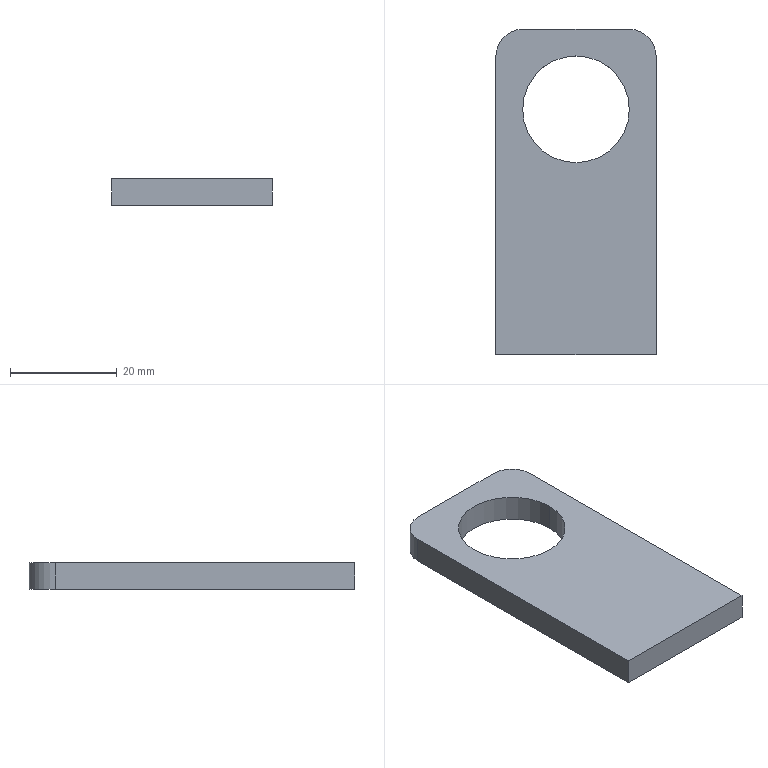Part | SolidWorks | features Extrusion 1, Fillet 1 | 1 solid | 10 faces | box 30 x 61 x 5 mm | volume 7526 mm3 | plane 6 | cylinder 4 | commonest cylinder face diameters 10 x2 20 x2
STEP:
#1=CARTESIAN_POINT('',(-10.,15.5,2.5));
#2=VERTEX_POINT('',#1);
#3=CARTESIAN_POINT('',(10.,15.5,2.5));
#4=VERTEX_POINT('',#3);
#5=CARTESIAN_POINT('',(0.,15.5,2.5));
#6=DIRECTION('',(0.,0.,1.));
#7=DIRECTION('',(1.,0.,0.));
#8=AXIS2_PLACEMENT_3D('',#5,#6,#7);
#9=CIRCLE('',#8,10.);
#10=EDGE_CURVE('',#2,#4,#9,.T.);
#11=ORIENTED_EDGE('',*,*,#10,.T.);
#12=CARTESIAN_POINT('',(10.,15.5,-2.5));
#13=VERTEX_POINT('',#12);
#14=CARTESIAN_POINT('',(10.,15.5,2.5));
#15=DIRECTION('',(0.,0.,-1.));
#16=VECTOR('',#15,1000.);
#17=LINE('',#14,#16);
#18=EDGE_CURVE('',#4,#13,#17,.T.);
#19=ORIENTED_EDGE('',*,*,#18,.T.);
#20=CARTESIAN_POINT('',(-10.,15.5,-2.5));
#21=VERTEX_POINT('',#20);
#22=CARTESIAN_POINT('',(0.,15.5,-2.5));
#23=DIRECTION('',(0.,0.,1.));
#24=DIRECTION('',(1.,0.,0.));
#25=AXIS2_PLACEMENT_3D('',#22,#23,#24);
#26=CIRCLE('',#25,10.);
#27=EDGE_CURVE('',#21,#13,#26,.T.);
#28=ORIENTED_EDGE('',*,*,#27,.F.);
#29=CARTESIAN_POINT('',(-10.,15.5,2.5));
#30=DIRECTION('',(0.,0.,-1.));
#31=VECTOR('',#30,1000.);
#32=LINE('',#29,#31);
#33=EDGE_CURVE('',#2,#21,#32,.T.);
#34=ORIENTED_EDGE('',*,*,#33,.F.);
#35=EDGE_LOOP('',(#11,#19,#28,#34));
#36=FACE_OUTER_BOUND('',#35,.T.);
#37=CARTESIAN_POINT('',(0.,15.5,2.5));
#38=DIRECTION('',(0.,0.,-1.));
#39=DIRECTION('',(-1.,0.,0.));
#40=AXIS2_PLACEMENT_3D('',#37,#38,#39);
#41=CYLINDRICAL_SURFACE('',#40,10.);
#42=ADVANCED_FACE('',(#36),#41,.F.);
#43=CARTESIAN_POINT('',(15.,-30.5,2.5));
#44=VERTEX_POINT('',#43);
#45=CARTESIAN_POINT('',(15.,25.5,2.5));
#46=VERTEX_POINT('',#45);
#47=CARTESIAN_POINT('',(15.,-30.5,2.5));
#48=DIRECTION('',(0.,1.,0.));
#49=VECTOR('',#48,1000.);
#50=LINE('',#47,#49);
#51=EDGE_CURVE('',#44,#46,#50,.T.);
#52=ORIENTED_EDGE('',*,*,#51,.T.);
#53=CARTESIAN_POINT('',(10.,30.5,2.5));
#54=VERTEX_POINT('',#53);
#55=CARTESIAN_POINT('',(10.,25.5,2.5));
#56=DIRECTION('',(0.,0.,1.));
#57=DIRECTION('',(-1.,0.,0.));
#58=AXIS2_PLACEMENT_3D('',#55,#56,#57);
#59=CIRCLE('',#58,5.);
#60=EDGE_CURVE('',#46,#54,#59,.T.);
#61=ORIENTED_EDGE('',*,*,#60,.T.);
#62=CARTESIAN_POINT('',(-10.,30.5,2.5));
#63=VERTEX_POINT('',#62);
#64=CARTESIAN_POINT('',(-15.,30.5,2.5));
#65=DIRECTION('',(-1.,0.,0.));
#66=VECTOR('',#65,1000.);
#67=LINE('',#64,#66);
#68=EDGE_CURVE('',#54,#63,#67,.T.);
#69=ORIENTED_EDGE('',*,*,#68,.T.);
#70=CARTESIAN_POINT('',(-15.,25.5,2.5));
#71=VERTEX_POINT('',#70);
#72=CARTESIAN_POINT('',(-10.,25.5,2.5));
#73=DIRECTION('',(0.,0.,1.));
#74=DIRECTION('',(-1.,0.,0.));
#75=AXIS2_PLACEMENT_3D('',#72,#73,#74);
#76=CIRCLE('',#75,5.);
#77=EDGE_CURVE('',#63,#71,#76,.T.);
#78=ORIENTED_EDGE('',*,*,#77,.T.);
#79=CARTESIAN_POINT('',(-15.,-30.5,2.5));
#80=VERTEX_POINT('',#79);
#81=CARTESIAN_POINT('',(-15.,-30.5,2.5));
#82=DIRECTION('',(0.,-1.,0.));
#83=VECTOR('',#82,1000.);
#84=LINE('',#81,#83);
#85=EDGE_CURVE('',#71,#80,#84,.T.);
#86=ORIENTED_EDGE('',*,*,#85,.T.);
#87=CARTESIAN_POINT('',(-15.,-30.5,2.5));
#88=DIRECTION('',(1.,0.,0.));
#89=VECTOR('',#88,1000.);
#90=LINE('',#87,#89);
#91=EDGE_CURVE('',#80,#44,#90,.T.);
#92=ORIENTED_EDGE('',*,*,#91,.T.);
#93=EDGE_LOOP('',(#52,#61,#69,#78,#86,#92));
#94=FACE_OUTER_BOUND('',#93,.T.);
#95=ORIENTED_EDGE('',*,*,#10,.F.);
#96=CARTESIAN_POINT('',(0.,15.5,2.5));
#97=DIRECTION('',(0.,0.,1.));
#98=DIRECTION('',(1.,0.,0.));
#99=AXIS2_PLACEMENT_3D('',#96,#97,#98);
#100=CIRCLE('',#99,10.);
#101=EDGE_CURVE('',#4,#2,#100,.T.);
#102=ORIENTED_EDGE('',*,*,#101,.F.);
#103=EDGE_LOOP('',(#95,#102));
#104=FACE_BOUND('',#103,.T.);
#105=CARTESIAN_POINT('',(0.,0.,2.5));
#106=DIRECTION('',(0.,0.,-1.));
#107=DIRECTION('',(-1.,0.,0.));
#108=AXIS2_PLACEMENT_3D('',#105,#106,#107);
#109=PLANE('',#108);
#110=ADVANCED_FACE('',(#94,#104),#109,.F.);
#111=CARTESIAN_POINT('',(10.,30.5,-2.5));
#112=VERTEX_POINT('',#111);
#113=CARTESIAN_POINT('',(-10.,30.5,-2.5));
#114=VERTEX_POINT('',#113);
#115=CARTESIAN_POINT('',(-15.,30.5,-2.5));
#116=DIRECTION('',(-1.,0.,0.));
#117=VECTOR('',#116,1000.);
#118=LINE('',#115,#117);
#119=EDGE_CURVE('',#112,#114,#118,.T.);
#120=ORIENTED_EDGE('',*,*,#119,.F.);
#121=CARTESIAN_POINT('',(15.,25.5,-2.5));
#122=VERTEX_POINT('',#121);
#123=CARTESIAN_POINT('',(10.,25.5,-2.5));
#124=DIRECTION('',(0.,0.,-1.));
#125=DIRECTION('',(-1.,0.,0.));
#126=AXIS2_PLACEMENT_3D('',#123,#124,#125);
#127=CIRCLE('',#126,5.);
#128=EDGE_CURVE('',#112,#122,#127,.T.);
#129=ORIENTED_EDGE('',*,*,#128,.T.);
#130=CARTESIAN_POINT('',(15.,-30.5,-2.5));
#131=VERTEX_POINT('',#130);
#132=CARTESIAN_POINT('',(15.,-30.5,-2.5));
#133=DIRECTION('',(0.,1.,0.));
#134=VECTOR('',#133,1000.);
#135=LINE('',#132,#134);
#136=EDGE_CURVE('',#131,#122,#135,.T.);
#137=ORIENTED_EDGE('',*,*,#136,.F.);
#138=CARTESIAN_POINT('',(-15.,-30.5,-2.5));
#139=VERTEX_POINT('',#138);
#140=CARTESIAN_POINT('',(-15.,-30.5,-2.5));
#141=DIRECTION('',(1.,0.,0.));
#142=VECTOR('',#141,1000.);
#143=LINE('',#140,#142);
#144=EDGE_CURVE('',#139,#131,#143,.T.);
#145=ORIENTED_EDGE('',*,*,#144,.F.);
#146=CARTESIAN_POINT('',(-15.,25.5,-2.5));
#147=VERTEX_POINT('',#146);
#148=CARTESIAN_POINT('',(-15.,-30.5,-2.5));
#149=DIRECTION('',(0.,-1.,0.));
#150=VECTOR('',#149,1000.);
#151=LINE('',#148,#150);
#152=EDGE_CURVE('',#147,#139,#151,.T.);
#153=ORIENTED_EDGE('',*,*,#152,.F.);
#154=CARTESIAN_POINT('',(-10.,25.5,-2.5));
#155=DIRECTION('',(0.,0.,-1.));
#156=DIRECTION('',(-1.,0.,0.));
#157=AXIS2_PLACEMENT_3D('',#154,#155,#156);
#158=CIRCLE('',#157,5.);
#159=EDGE_CURVE('',#147,#114,#158,.T.);
#160=ORIENTED_EDGE('',*,*,#159,.T.);
#161=EDGE_LOOP('',(#120,#129,#137,#145,#153,#160));
#162=FACE_OUTER_BOUND('',#161,.T.);
#163=ORIENTED_EDGE('',*,*,#27,.T.);
#164=CARTESIAN_POINT('',(0.,15.5,-2.5));
#165=DIRECTION('',(0.,0.,1.));
#166=DIRECTION('',(1.,0.,0.));
#167=AXIS2_PLACEMENT_3D('',#164,#165,#166);
#168=CIRCLE('',#167,10.);
#169=EDGE_CURVE('',#13,#21,#168,.T.);
#170=ORIENTED_EDGE('',*,*,#169,.T.);
#171=EDGE_LOOP('',(#163,#170));
#172=FACE_BOUND('',#171,.T.);
#173=CARTESIAN_POINT('',(0.,0.,-2.5));
#174=DIRECTION('',(0.,0.,-1.));
#175=DIRECTION('',(-1.,0.,0.));
#176=AXIS2_PLACEMENT_3D('',#173,#174,#175);
#177=PLANE('',#176);
#178=ADVANCED_FACE('',(#162,#172),#177,.T.);
#179=ORIENTED_EDGE('',*,*,#136,.T.);
#180=CARTESIAN_POINT('',(15.,25.5,2.5));
#181=DIRECTION('',(0.,0.,1.));
#182=VECTOR('',#181,1000.);
#183=LINE('',#180,#182);
#184=EDGE_CURVE('',#122,#46,#183,.T.);
#185=ORIENTED_EDGE('',*,*,#184,.T.);
#186=ORIENTED_EDGE('',*,*,#51,.F.);
#187=CARTESIAN_POINT('',(15.,-30.5,2.5));
#188=DIRECTION('',(0.,0.,-1.));
#189=VECTOR('',#188,1000.);
#190=LINE('',#187,#189);
#191=EDGE_CURVE('',#44,#131,#190,.T.);
#192=ORIENTED_EDGE('',*,*,#191,.T.);
#193=EDGE_LOOP('',(#179,#185,#186,#192));
#194=FACE_OUTER_BOUND('',#193,.T.);
#195=CARTESIAN_POINT('',(15.,-30.5,2.5));
#196=DIRECTION('',(-1.,0.,0.));
#197=DIRECTION('',(0.,0.,1.));
#198=AXIS2_PLACEMENT_3D('',#195,#196,#197);
#199=PLANE('',#198);
#200=ADVANCED_FACE('',(#194),#199,.F.);
#201=ORIENTED_EDGE('',*,*,#68,.F.);
#202=CARTESIAN_POINT('',(10.,30.5,2.5));
#203=DIRECTION('',(0.,0.,-1.));
#204=VECTOR('',#203,1000.);
#205=LINE('',#202,#204);
#206=EDGE_CURVE('',#54,#112,#205,.T.);
#207=ORIENTED_EDGE('',*,*,#206,.T.);
#208=ORIENTED_EDGE('',*,*,#119,.T.);
#209=CARTESIAN_POINT('',(-10.,30.5,2.5));
#210=DIRECTION('',(0.,0.,1.));
#211=VECTOR('',#210,1000.);
#212=LINE('',#209,#211);
#213=EDGE_CURVE('',#114,#63,#212,.T.);
#214=ORIENTED_EDGE('',*,*,#213,.T.);
#215=EDGE_LOOP('',(#201,#207,#208,#214));
#216=FACE_OUTER_BOUND('',#215,.T.);
#217=CARTESIAN_POINT('',(-15.,30.5,2.5));
#218=DIRECTION('',(0.,-1.,0.));
#219=DIRECTION('',(0.,0.,-1.));
#220=AXIS2_PLACEMENT_3D('',#217,#218,#219);
#221=PLANE('',#220);
#222=ADVANCED_FACE('',(#216),#221,.F.);
#223=ORIENTED_EDGE('',*,*,#85,.F.);
#224=CARTESIAN_POINT('',(-15.,25.5,2.5));
#225=DIRECTION('',(0.,0.,-1.));
#226=VECTOR('',#225,1000.);
#227=LINE('',#224,#226);
#228=EDGE_CURVE('',#71,#147,#227,.T.);
#229=ORIENTED_EDGE('',*,*,#228,.T.);
#230=ORIENTED_EDGE('',*,*,#152,.T.);
#231=CARTESIAN_POINT('',(-15.,-30.5,2.5));
#232=DIRECTION('',(0.,0.,-1.));
#233=VECTOR('',#232,1000.);
#234=LINE('',#231,#233);
#235=EDGE_CURVE('',#80,#139,#234,.T.);
#236=ORIENTED_EDGE('',*,*,#235,.F.);
#237=EDGE_LOOP('',(#223,#229,#230,#236));
#238=FACE_OUTER_BOUND('',#237,.T.);
#239=CARTESIAN_POINT('',(-15.,-30.5,2.5));
#240=DIRECTION('',(1.,0.,0.));
#241=DIRECTION('',(0.,0.,-1.));
#242=AXIS2_PLACEMENT_3D('',#239,#240,#241);
#243=PLANE('',#242);
#244=ADVANCED_FACE('',(#238),#243,.F.);
#245=ORIENTED_EDGE('',*,*,#144,.T.);
#246=ORIENTED_EDGE('',*,*,#191,.F.);
#247=ORIENTED_EDGE('',*,*,#91,.F.);
#248=ORIENTED_EDGE('',*,*,#235,.T.);
#249=EDGE_LOOP('',(#245,#246,#247,#248));
#250=FACE_OUTER_BOUND('',#249,.T.);
#251=CARTESIAN_POINT('',(-15.,-30.5,2.5));
#252=DIRECTION('',(0.,1.,0.));
#253=DIRECTION('',(0.,0.,1.));
#254=AXIS2_PLACEMENT_3D('',#251,#252,#253);
#255=PLANE('',#254);
#256=ADVANCED_FACE('',(#250),#255,.F.);
#257=ORIENTED_EDGE('',*,*,#18,.F.);
#258=ORIENTED_EDGE('',*,*,#101,.T.);
#259=ORIENTED_EDGE('',*,*,#33,.T.);
#260=ORIENTED_EDGE('',*,*,#169,.F.);
#261=EDGE_LOOP('',(#257,#258,#259,#260));
#262=FACE_OUTER_BOUND('',#261,.T.);
#263=CARTESIAN_POINT('',(0.,15.5,2.5));
#264=DIRECTION('',(0.,0.,-1.));
#265=DIRECTION('',(-1.,0.,0.));
#266=AXIS2_PLACEMENT_3D('',#263,#264,#265);
#267=CYLINDRICAL_SURFACE('',#266,10.);
#268=ADVANCED_FACE('',(#262),#267,.F.);
#269=ORIENTED_EDGE('',*,*,#60,.F.);
#270=ORIENTED_EDGE('',*,*,#184,.F.);
#271=ORIENTED_EDGE('',*,*,#128,.F.);
#272=ORIENTED_EDGE('',*,*,#206,.F.);
#273=EDGE_LOOP('',(#269,#270,#271,#272));
#274=FACE_OUTER_BOUND('',#273,.T.);
#275=CARTESIAN_POINT('',(10.,25.5,2.5));
#276=DIRECTION('',(0.,0.,-1.));
#277=DIRECTION('',(-1.,0.,0.));
#278=AXIS2_PLACEMENT_3D('',#275,#276,#277);
#279=CYLINDRICAL_SURFACE('',#278,5.);
#280=ADVANCED_FACE('',(#274),#279,.T.);
#281=ORIENTED_EDGE('',*,*,#77,.F.);
#282=ORIENTED_EDGE('',*,*,#213,.F.);
#283=ORIENTED_EDGE('',*,*,#159,.F.);
#284=ORIENTED_EDGE('',*,*,#228,.F.);
#285=EDGE_LOOP('',(#281,#282,#283,#284));
#286=FACE_OUTER_BOUND('',#285,.T.);
#287=CARTESIAN_POINT('',(-10.,25.5,2.5));
#288=DIRECTION('',(0.,0.,-1.));
#289=DIRECTION('',(-1.,0.,0.));
#290=AXIS2_PLACEMENT_3D('',#287,#288,#289);
#291=CYLINDRICAL_SURFACE('',#290,5.);
#292=ADVANCED_FACE('',(#286),#291,.T.);
#293=CLOSED_SHELL('',(#42,#110,#178,#200,#222,#244,#256,#268,#280,#292));
#294=MANIFOLD_SOLID_BREP('',#293);
#295=CARTESIAN_POINT('',(0.,0.,0.));
#296=DIRECTION('',(0.,0.,1.));
#297=DIRECTION('',(1.,0.,0.));
#298=AXIS2_PLACEMENT_3D('',#295,#296,#297);
#299=(LENGTH_UNIT()NAMED_UNIT(*)SI_UNIT(.MILLI.,.METRE.));
#300=UNCERTAINTY_MEASURE_WITH_UNIT(LENGTH_MEASURE(0.00001),#299,'','');
#301=(NAMED_UNIT(*)PLANE_ANGLE_UNIT()SI_UNIT($,.RADIAN.));
#302=(NAMED_UNIT(*)SI_UNIT($,.STERADIAN.)SOLID_ANGLE_UNIT());
#303=(GEOMETRIC_REPRESENTATION_CONTEXT(3)GLOBAL_UNCERTAINTY_ASSIGNED_CONTEXT((#300))GLOBAL_UNIT_ASSIGNED_CONTEXT((#299,#301,#302))REPRESENTATION_CONTEXT('',''));
#304=ADVANCED_BREP_SHAPE_REPRESENTATION('',(#294,#298),#303);